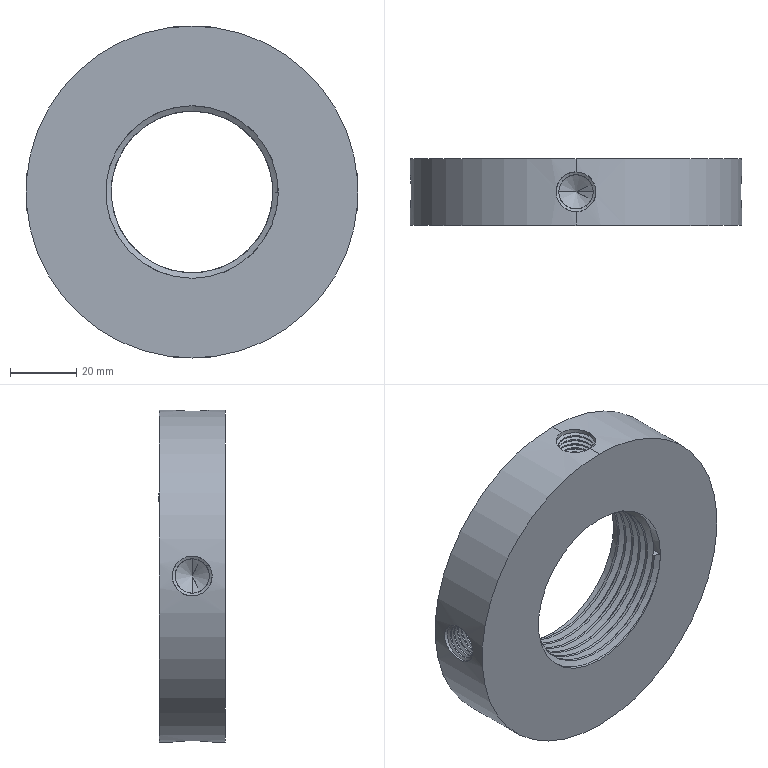Part | SolidWorks | features CirPattern 2, HoleWzd 2, SweepThread 2, 3DProfileFeature 1, Extrusion 1 | 1 solid | 137 faces | box 100 x 20.124 x 100 mm | volume 110228 mm3 | cylinder 101 | spline 16 | plane 12 | cone 8 | commonest cylinder face diameters 12 x84 52 x15 100 x2